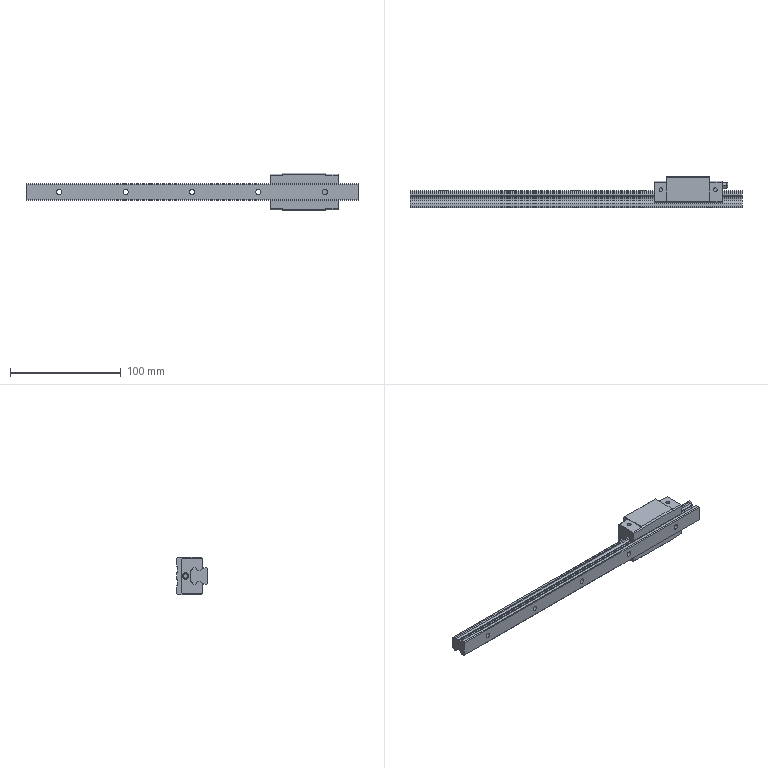Part | SolidWorks | 2 solids | 199 faces | box 300 x 28 x 34 mm | volume 92053 mm3 | plane 96 | cylinder 85 | cone 16 | torus 2 | commonest cylinder face diameters 0.8 x15 4.5 x10 7.5 x10 3.24 x8 3.242 x8 3.3 x8